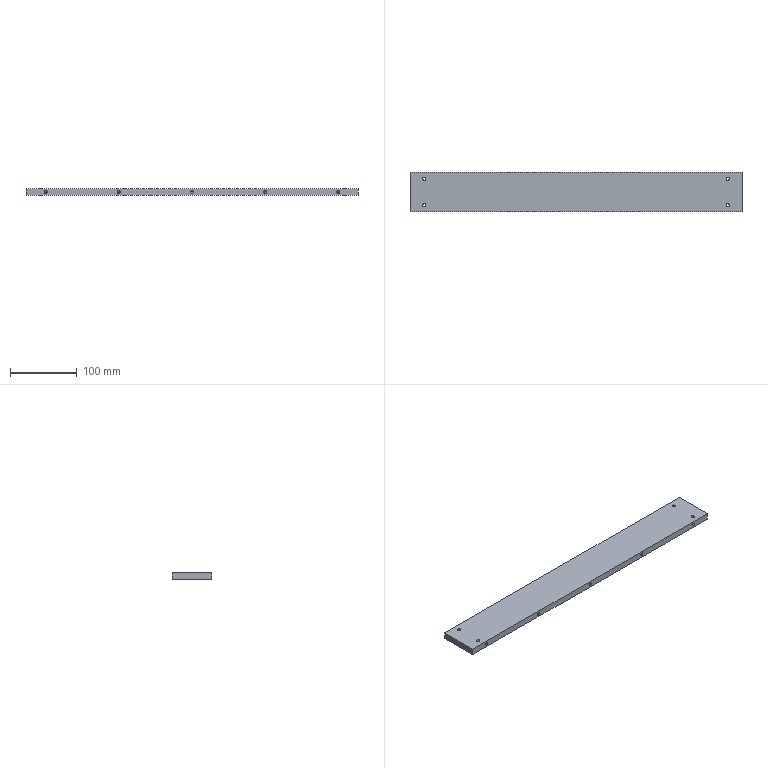Part | SolidWorks | features HoleWzd 3, Extrusion 1 | 1 solid | 54 faces | box 499 x 60 x 10 mm | volume 297280 mm3 | cylinder 28 | cone 20 | plane 6 | commonest cylinder face diameters 3.3 x10 4.2 x10 5 x8
STEP:
#1=CARTESIAN_POINT('',(0.,49.9,-1.65));
#2=VERTEX_POINT('',#1);
#3=CARTESIAN_POINT('',(0.,49.9,1.65));
#4=VERTEX_POINT('',#3);
#5=CARTESIAN_POINT('',(0.,49.9,0.));
#6=DIRECTION('',(0.,1.,0.));
#7=DIRECTION('',(0.,0.,1.));
#8=AXIS2_PLACEMENT_3D('',#5,#6,#7);
#9=CIRCLE('',#8,1.65);
#10=EDGE_CURVE('',#2,#4,#9,.T.);
#11=ORIENTED_EDGE('',*,*,#10,.F.);
#12=CARTESIAN_POINT('',(0.,60.,-1.65));
#13=VERTEX_POINT('',#12);
#14=CARTESIAN_POINT('',(0.,60.,-1.65));
#15=DIRECTION('',(0.,1.,0.));
#16=VECTOR('',#15,1000.);
#17=LINE('',#14,#16);
#18=EDGE_CURVE('',#2,#13,#17,.T.);
#19=ORIENTED_EDGE('',*,*,#18,.T.);
#20=CARTESIAN_POINT('',(0.,60.,1.65));
#21=VERTEX_POINT('',#20);
#22=CARTESIAN_POINT('',(0.,60.,0.));
#23=DIRECTION('',(0.,1.,0.));
#24=DIRECTION('',(0.,0.,1.));
#25=AXIS2_PLACEMENT_3D('',#22,#23,#24);
#26=CIRCLE('',#25,1.65);
#27=EDGE_CURVE('',#13,#21,#26,.T.);
#28=ORIENTED_EDGE('',*,*,#27,.T.);
#29=CARTESIAN_POINT('',(0.,60.,1.65));
#30=DIRECTION('',(0.,1.,0.));
#31=VECTOR('',#30,1000.);
#32=LINE('',#29,#31);
#33=EDGE_CURVE('',#4,#21,#32,.T.);
#34=ORIENTED_EDGE('',*,*,#33,.F.);
#35=EDGE_LOOP('',(#11,#19,#28,#34));
#36=FACE_OUTER_BOUND('',#35,.T.);
#37=CARTESIAN_POINT('',(0.,60.,0.));
#38=DIRECTION('',(0.,1.,0.));
#39=DIRECTION('',(0.,0.,1.));
#40=AXIS2_PLACEMENT_3D('',#37,#38,#39);
#41=CYLINDRICAL_SURFACE('',#40,1.65);
#42=ADVANCED_FACE('',(#36),#41,.F.);
#43=CARTESIAN_POINT('',(0.,48.909,0.));
#44=VERTEX_POINT('',#43);
#45=CARTESIAN_POINT('',(0.,49.9,1.65));
#46=DIRECTION('',(0.,0.515,0.8572));
#47=VECTOR('',#46,1000.);
#48=LINE('',#45,#47);
#49=EDGE_CURVE('',#44,#4,#48,.T.);
#50=ORIENTED_EDGE('',*,*,#49,.F.);
#51=CARTESIAN_POINT('',(0.,49.9,-1.65));
#52=DIRECTION('',(0.,0.515,-0.8572));
#53=VECTOR('',#52,1000.);
#54=LINE('',#51,#53);
#55=EDGE_CURVE('',#44,#2,#54,.T.);
#56=ORIENTED_EDGE('',*,*,#55,.T.);
#57=ORIENTED_EDGE('',*,*,#10,.T.);
#58=EDGE_LOOP('',(#50,#56,#57));
#59=FACE_OUTER_BOUND('',#58,.T.);
#60=CARTESIAN_POINT('',(0.,49.9,0.));
#61=DIRECTION('',(0.,1.,0.));
#62=DIRECTION('',(0.,0.,1.));
#63=AXIS2_PLACEMENT_3D('',#60,#61,#62);
#64=CONICAL_SURFACE('',#63,1.65,1.03);
#65=ADVANCED_FACE('',(#59),#64,.F.);
#66=CARTESIAN_POINT('',(-175.,49.9,-1.65));
#67=VERTEX_POINT('',#66);
#68=CARTESIAN_POINT('',(-175.,49.9,1.65));
#69=VERTEX_POINT('',#68);
#70=CARTESIAN_POINT('',(-175.,49.9,0.));
#71=DIRECTION('',(0.,1.,0.));
#72=DIRECTION('',(0.,0.,1.));
#73=AXIS2_PLACEMENT_3D('',#70,#71,#72);
#74=CIRCLE('',#73,1.65);
#75=EDGE_CURVE('',#67,#69,#74,.T.);
#76=ORIENTED_EDGE('',*,*,#75,.F.);
#77=CARTESIAN_POINT('',(-175.,60.,-1.65));
#78=VERTEX_POINT('',#77);
#79=CARTESIAN_POINT('',(-175.,60.,-1.65));
#80=DIRECTION('',(0.,1.,0.));
#81=VECTOR('',#80,1000.);
#82=LINE('',#79,#81);
#83=EDGE_CURVE('',#67,#78,#82,.T.);
#84=ORIENTED_EDGE('',*,*,#83,.T.);
#85=CARTESIAN_POINT('',(-175.,60.,1.65));
#86=VERTEX_POINT('',#85);
#87=CARTESIAN_POINT('',(-175.,60.,0.));
#88=DIRECTION('',(0.,1.,0.));
#89=DIRECTION('',(0.,0.,1.));
#90=AXIS2_PLACEMENT_3D('',#87,#88,#89);
#91=CIRCLE('',#90,1.65);
#92=EDGE_CURVE('',#78,#86,#91,.T.);
#93=ORIENTED_EDGE('',*,*,#92,.T.);
#94=CARTESIAN_POINT('',(-175.,60.,1.65));
#95=DIRECTION('',(0.,1.,0.));
#96=VECTOR('',#95,1000.);
#97=LINE('',#94,#96);
#98=EDGE_CURVE('',#69,#86,#97,.T.);
#99=ORIENTED_EDGE('',*,*,#98,.F.);
#100=EDGE_LOOP('',(#76,#84,#93,#99));
#101=FACE_OUTER_BOUND('',#100,.T.);
#102=CARTESIAN_POINT('',(-175.,60.,0.));
#103=DIRECTION('',(0.,1.,0.));
#104=DIRECTION('',(0.,0.,1.));
#105=AXIS2_PLACEMENT_3D('',#102,#103,#104);
#106=CYLINDRICAL_SURFACE('',#105,1.65);
#107=ADVANCED_FACE('',(#101),#106,.F.);
#108=CARTESIAN_POINT('',(-175.,48.909,0.));
#109=VERTEX_POINT('',#108);
#110=CARTESIAN_POINT('',(-175.,49.9,1.65));
#111=DIRECTION('',(0.,0.515,0.8572));
#112=VECTOR('',#111,1000.);
#113=LINE('',#110,#112);
#114=EDGE_CURVE('',#109,#69,#113,.T.);
#115=ORIENTED_EDGE('',*,*,#114,.F.);
#116=CARTESIAN_POINT('',(-175.,49.9,-1.65));
#117=DIRECTION('',(0.,0.515,-0.8572));
#118=VECTOR('',#117,1000.);
#119=LINE('',#116,#118);
#120=EDGE_CURVE('',#109,#67,#119,.T.);
#121=ORIENTED_EDGE('',*,*,#120,.T.);
#122=ORIENTED_EDGE('',*,*,#75,.T.);
#123=EDGE_LOOP('',(#115,#121,#122));
#124=FACE_OUTER_BOUND('',#123,.T.);
#125=CARTESIAN_POINT('',(-175.,49.9,0.));
#126=DIRECTION('',(0.,1.,0.));
#127=DIRECTION('',(0.,0.,1.));
#128=AXIS2_PLACEMENT_3D('',#125,#126,#127);
#129=CONICAL_SURFACE('',#128,1.65,1.03);
#130=ADVANCED_FACE('',(#124),#129,.F.);
#131=CARTESIAN_POINT('',(175.,49.9,-1.65));
#132=VERTEX_POINT('',#131);
#133=CARTESIAN_POINT('',(175.,49.9,1.65));
#134=VERTEX_POINT('',#133);
#135=CARTESIAN_POINT('',(175.,49.9,0.));
#136=DIRECTION('',(0.,1.,0.));
#137=DIRECTION('',(0.,0.,1.));
#138=AXIS2_PLACEMENT_3D('',#135,#136,#137);
#139=CIRCLE('',#138,1.65);
#140=EDGE_CURVE('',#132,#134,#139,.T.);
#141=ORIENTED_EDGE('',*,*,#140,.F.);
#142=CARTESIAN_POINT('',(175.,60.,-1.65));
#143=VERTEX_POINT('',#142);
#144=CARTESIAN_POINT('',(175.,60.,-1.65));
#145=DIRECTION('',(0.,1.,0.));
#146=VECTOR('',#145,1000.);
#147=LINE('',#144,#146);
#148=EDGE_CURVE('',#132,#143,#147,.T.);
#149=ORIENTED_EDGE('',*,*,#148,.T.);
#150=CARTESIAN_POINT('',(175.,60.,1.65));
#151=VERTEX_POINT('',#150);
#152=CARTESIAN_POINT('',(175.,60.,0.));
#153=DIRECTION('',(0.,1.,0.));
#154=DIRECTION('',(0.,0.,1.));
#155=AXIS2_PLACEMENT_3D('',#152,#153,#154);
#156=CIRCLE('',#155,1.65);
#157=EDGE_CURVE('',#143,#151,#156,.T.);
#158=ORIENTED_EDGE('',*,*,#157,.T.);
#159=CARTESIAN_POINT('',(175.,60.,1.65));
#160=DIRECTION('',(0.,1.,0.));
#161=VECTOR('',#160,1000.);
#162=LINE('',#159,#161);
#163=EDGE_CURVE('',#134,#151,#162,.T.);
#164=ORIENTED_EDGE('',*,*,#163,.F.);
#165=EDGE_LOOP('',(#141,#149,#158,#164));
#166=FACE_OUTER_BOUND('',#165,.T.);
#167=CARTESIAN_POINT('',(175.,60.,0.));
#168=DIRECTION('',(0.,1.,0.));
#169=DIRECTION('',(0.,0.,1.));
#170=AXIS2_PLACEMENT_3D('',#167,#168,#169);
#171=CYLINDRICAL_SURFACE('',#170,1.65);
#172=ADVANCED_FACE('',(#166),#171,.F.);
#173=CARTESIAN_POINT('',(175.,48.909,0.));
#174=VERTEX_POINT('',#173);
#175=CARTESIAN_POINT('',(175.,49.9,1.65));
#176=DIRECTION('',(0.,0.515,0.8572));
#177=VECTOR('',#176,1000.);
#178=LINE('',#175,#177);
#179=EDGE_CURVE('',#174,#134,#178,.T.);
#180=ORIENTED_EDGE('',*,*,#179,.F.);
#181=CARTESIAN_POINT('',(175.,49.9,-1.65));
#182=DIRECTION('',(0.,0.515,-0.8572));
#183=VECTOR('',#182,1000.);
#184=LINE('',#181,#183);
#185=EDGE_CURVE('',#174,#132,#184,.T.);
#186=ORIENTED_EDGE('',*,*,#185,.T.);
#187=ORIENTED_EDGE('',*,*,#140,.T.);
#188=EDGE_LOOP('',(#180,#186,#187));
#189=FACE_OUTER_BOUND('',#188,.T.);
#190=CARTESIAN_POINT('',(175.,49.9,0.));
#191=DIRECTION('',(0.,1.,0.));
#192=DIRECTION('',(0.,0.,1.));
#193=AXIS2_PLACEMENT_3D('',#190,#191,#192);
#194=CONICAL_SURFACE('',#193,1.65,1.03);
#195=ADVANCED_FACE('',(#189),#194,.F.);
#196=CARTESIAN_POINT('',(-160.,49.9,-1.65));
#197=VERTEX_POINT('',#196);
#198=CARTESIAN_POINT('',(-160.,49.9,1.65));
#199=VERTEX_POINT('',#198);
#200=CARTESIAN_POINT('',(-160.,49.9,0.));
#201=DIRECTION('',(0.,1.,0.));
#202=DIRECTION('',(0.,0.,1.));
#203=AXIS2_PLACEMENT_3D('',#200,#201,#202);
#204=CIRCLE('',#203,1.65);
#205=EDGE_CURVE('',#197,#199,#204,.T.);
#206=ORIENTED_EDGE('',*,*,#205,.F.);
#207=CARTESIAN_POINT('',(-160.,60.,-1.65));
#208=VERTEX_POINT('',#207);
#209=CARTESIAN_POINT('',(-160.,60.,-1.65));
#210=DIRECTION('',(0.,1.,0.));
#211=VECTOR('',#210,1000.);
#212=LINE('',#209,#211);
#213=EDGE_CURVE('',#197,#208,#212,.T.);
#214=ORIENTED_EDGE('',*,*,#213,.T.);
#215=CARTESIAN_POINT('',(-160.,60.,1.65));
#216=VERTEX_POINT('',#215);
#217=CARTESIAN_POINT('',(-160.,60.,0.));
#218=DIRECTION('',(0.,1.,0.));
#219=DIRECTION('',(0.,0.,1.));
#220=AXIS2_PLACEMENT_3D('',#217,#218,#219);
#221=CIRCLE('',#220,1.65);
#222=EDGE_CURVE('',#208,#216,#221,.T.);
#223=ORIENTED_EDGE('',*,*,#222,.T.);
#224=CARTESIAN_POINT('',(-160.,60.,1.65));
#225=DIRECTION('',(0.,1.,0.));
#226=VECTOR('',#225,1000.);
#227=LINE('',#224,#226);
#228=EDGE_CURVE('',#199,#216,#227,.T.);
#229=ORIENTED_EDGE('',*,*,#228,.F.);
#230=EDGE_LOOP('',(#206,#214,#223,#229));
#231=FACE_OUTER_BOUND('',#230,.T.);
#232=CARTESIAN_POINT('',(-160.,60.,0.));
#233=DIRECTION('',(0.,1.,0.));
#234=DIRECTION('',(0.,0.,1.));
#235=AXIS2_PLACEMENT_3D('',#232,#233,#234);
#236=CYLINDRICAL_SURFACE('',#235,1.65);
#237=ADVANCED_FACE('',(#231),#236,.F.);
#238=CARTESIAN_POINT('',(-160.,48.909,0.));
#239=VERTEX_POINT('',#238);
#240=CARTESIAN_POINT('',(-160.,49.9,1.65));
#241=DIRECTION('',(0.,0.515,0.8572));
#242=VECTOR('',#241,1000.);
#243=LINE('',#240,#242);
#244=EDGE_CURVE('',#239,#199,#243,.T.);
#245=ORIENTED_EDGE('',*,*,#244,.F.);
#246=CARTESIAN_POINT('',(-160.,49.9,-1.65));
#247=DIRECTION('',(0.,0.515,-0.8572));
#248=VECTOR('',#247,1000.);
#249=LINE('',#246,#248);
#250=EDGE_CURVE('',#239,#197,#249,.T.);
#251=ORIENTED_EDGE('',*,*,#250,.T.);
#252=ORIENTED_EDGE('',*,*,#205,.T.);
#253=EDGE_LOOP('',(#245,#251,#252));
#254=FACE_OUTER_BOUND('',#253,.T.);
#255=CARTESIAN_POINT('',(-160.,49.9,0.));
#256=DIRECTION('',(0.,1.,0.));
#257=DIRECTION('',(0.,0.,1.));
#258=AXIS2_PLACEMENT_3D('',#255,#256,#257);
#259=CONICAL_SURFACE('',#258,1.65,1.03);
#260=ADVANCED_FACE('',(#254),#259,.F.);
#261=CARTESIAN_POINT('',(160.,49.9,-1.65));
#262=VERTEX_POINT('',#261);
#263=CARTESIAN_POINT('',(160.,49.9,1.65));
#264=VERTEX_POINT('',#263);
#265=CARTESIAN_POINT('',(160.,49.9,0.));
#266=DIRECTION('',(0.,1.,0.));
#267=DIRECTION('',(0.,0.,1.));
#268=AXIS2_PLACEMENT_3D('',#265,#266,#267);
#269=CIRCLE('',#268,1.65);
#270=EDGE_CURVE('',#262,#264,#269,.T.);
#271=ORIENTED_EDGE('',*,*,#270,.F.);
#272=CARTESIAN_POINT('',(160.,60.,-1.65));
#273=VERTEX_POINT('',#272);
#274=CARTESIAN_POINT('',(160.,60.,-1.65));
#275=DIRECTION('',(0.,1.,0.));
#276=VECTOR('',#275,1000.);
#277=LINE('',#274,#276);
#278=EDGE_CURVE('',#262,#273,#277,.T.);
#279=ORIENTED_EDGE('',*,*,#278,.T.);
#280=CARTESIAN_POINT('',(160.,60.,1.65));
#281=VERTEX_POINT('',#280);
#282=CARTESIAN_POINT('',(160.,60.,0.));
#283=DIRECTION('',(0.,1.,0.));
#284=DIRECTION('',(0.,0.,1.));
#285=AXIS2_PLACEMENT_3D('',#282,#283,#284);
#286=CIRCLE('',#285,1.65);
#287=EDGE_CURVE('',#273,#281,#286,.T.);
#288=ORIENTED_EDGE('',*,*,#287,.T.);
#289=CARTESIAN_POINT('',(160.,60.,1.65));
#290=DIRECTION('',(0.,1.,0.));
#291=VECTOR('',#290,1000.);
#292=LINE('',#289,#291);
#293=EDGE_CURVE('',#264,#281,#292,.T.);
#294=ORIENTED_EDGE('',*,*,#293,.F.);
#295=EDGE_LOOP('',(#271,#279,#288,#294));
#296=FACE_OUTER_BOUND('',#295,.T.);
#297=CARTESIAN_POINT('',(160.,60.,0.));
#298=DIRECTION('',(0.,1.,0.));
#299=DIRECTION('',(0.,0.,1.));
#300=AXIS2_PLACEMENT_3D('',#297,#298,#299);
#301=CYLINDRICAL_SURFACE('',#300,1.65);
#302=ADVANCED_FACE('',(#296),#301,.F.);
#303=CARTESIAN_POINT('',(160.,48.909,0.));
#304=VERTEX_POINT('',#303);
#305=CARTESIAN_POINT('',(160.,49.9,1.65));
#306=DIRECTION('',(0.,0.515,0.8572));
#307=VECTOR('',#306,1000.);
#308=LINE('',#305,#307);
#309=EDGE_CURVE('',#304,#264,#308,.T.);
#310=ORIENTED_EDGE('',*,*,#309,.F.);
#311=CARTESIAN_POINT('',(160.,49.9,-1.65));
#312=DIRECTION('',(0.,0.515,-0.8572));
#313=VECTOR('',#312,1000.);
#314=LINE('',#311,#313);
#315=EDGE_CURVE('',#304,#262,#314,.T.);
#316=ORIENTED_EDGE('',*,*,#315,.T.);
#317=ORIENTED_EDGE('',*,*,#270,.T.);
#318=EDGE_LOOP('',(#310,#316,#317));
#319=FACE_OUTER_BOUND('',#318,.T.);
#320=CARTESIAN_POINT('',(160.,49.9,0.));
#321=DIRECTION('',(0.,1.,0.));
#322=DIRECTION('',(0.,0.,1.));
#323=AXIS2_PLACEMENT_3D('',#320,#321,#322);
#324=CONICAL_SURFACE('',#323,1.65,1.03);
#325=ADVANCED_FACE('',(#319),#324,.F.);
#326=CARTESIAN_POINT('',(225.5,50.,-5.));
#327=VERTEX_POINT('',#326);
#328=CARTESIAN_POINT('',(230.5,50.,-5.));
#329=VERTEX_POINT('',#328);
#330=CARTESIAN_POINT('',(228.,50.,-5.));
#331=DIRECTION('',(0.,0.,1.));
#332=DIRECTION('',(1.,0.,0.));
#333=AXIS2_PLACEMENT_3D('',#330,#331,#332);
#334=CIRCLE('',#333,2.5);
#335=EDGE_CURVE('',#327,#329,#334,.T.);
#336=ORIENTED_EDGE('',*,*,#335,.F.);
#337=CARTESIAN_POINT('',(225.5,50.,5.));
#338=VERTEX_POINT('',#337);
#339=CARTESIAN_POINT('',(225.5,50.,5.));
#340=DIRECTION('',(0.,0.,1.));
#341=VECTOR('',#340,1000.);
#342=LINE('',#339,#341);
#343=EDGE_CURVE('',#327,#338,#342,.T.);
#344=ORIENTED_EDGE('',*,*,#343,.T.);
#345=CARTESIAN_POINT('',(230.5,50.,5.));
#346=VERTEX_POINT('',#345);
#347=CARTESIAN_POINT('',(228.,50.,5.));
#348=DIRECTION('',(0.,0.,1.));
#349=DIRECTION('',(1.,0.,0.));
#350=AXIS2_PLACEMENT_3D('',#347,#348,#349);
#351=CIRCLE('',#350,2.5);
#352=EDGE_CURVE('',#338,#346,#351,.T.);
#353=ORIENTED_EDGE('',*,*,#352,.T.);
#354=CARTESIAN_POINT('',(230.5,50.,5.));
#355=DIRECTION('',(0.,0.,1.));
#356=VECTOR('',#355,1000.);
#357=LINE('',#354,#356);
#358=EDGE_CURVE('',#329,#346,#357,.T.);
#359=ORIENTED_EDGE('',*,*,#358,.F.);
#360=EDGE_LOOP('',(#336,#344,#353,#359));
#361=FACE_OUTER_BOUND('',#360,.T.);
#362=CARTESIAN_POINT('',(228.,50.,5.));
#363=DIRECTION('',(0.,0.,1.));
#364=DIRECTION('',(1.,0.,0.));
#365=AXIS2_PLACEMENT_3D('',#362,#363,#364);
#366=CYLINDRICAL_SURFACE('',#365,2.5);
#367=ADVANCED_FACE('',(#361),#366,.F.);
#368=CARTESIAN_POINT('',(225.5,10.,-5.));
#369=VERTEX_POINT('',#368);
#370=CARTESIAN_POINT('',(230.5,10.,-5.));
#371=VERTEX_POINT('',#370);
#372=CARTESIAN_POINT('',(228.,10.,-5.));
#373=DIRECTION('',(0.,0.,1.));
#374=DIRECTION('',(1.,0.,0.));
#375=AXIS2_PLACEMENT_3D('',#372,#373,#374);
#376=CIRCLE('',#375,2.5);
#377=EDGE_CURVE('',#369,#371,#376,.T.);
#378=ORIENTED_EDGE('',*,*,#377,.F.);
#379=CARTESIAN_POINT('',(225.5,10.,5.));
#380=VERTEX_POINT('',#379);
#381=CARTESIAN_POINT('',(225.5,10.,5.));
#382=DIRECTION('',(0.,0.,1.));
#383=VECTOR('',#382,1000.);
#384=LINE('',#381,#383);
#385=EDGE_CURVE('',#369,#380,#384,.T.);
#386=ORIENTED_EDGE('',*,*,#385,.T.);
#387=CARTESIAN_POINT('',(230.5,10.,5.));
#388=VERTEX_POINT('',#387);
#389=CARTESIAN_POINT('',(228.,10.,5.));
#390=DIRECTION('',(0.,0.,1.));
#391=DIRECTION('',(1.,0.,0.));
#392=AXIS2_PLACEMENT_3D('',#389,#390,#391);
#393=CIRCLE('',#392,2.5);
#394=EDGE_CURVE('',#380,#388,#393,.T.);
#395=ORIENTED_EDGE('',*,*,#394,.T.);
#396=CARTESIAN_POINT('',(230.5,10.,5.));
#397=DIRECTION('',(0.,0.,1.));
#398=VECTOR('',#397,1000.);
#399=LINE('',#396,#398);
#400=EDGE_CURVE('',#371,#388,#399,.T.);
#401=ORIENTED_EDGE('',*,*,#400,.F.);
#402=EDGE_LOOP('',(#378,#386,#395,#401));
#403=FACE_OUTER_BOUND('',#402,.T.);
#404=CARTESIAN_POINT('',(228.,10.,5.));
#405=DIRECTION('',(0.,0.,1.));
#406=DIRECTION('',(1.,0.,0.));
#407=AXIS2_PLACEMENT_3D('',#404,#405,#406);
#408=CYLINDRICAL_SURFACE('',#407,2.5);
#409=ADVANCED_FACE('',(#403),#408,.F.);
#410=CARTESIAN_POINT('',(-230.5,10.,-5.));
#411=VERTEX_POINT('',#410);
#412=CARTESIAN_POINT('',(-225.5,10.,-5.));
#413=VERTEX_POINT('',#412);
#414=CARTESIAN_POINT('',(-228.,10.,-5.));
#415=DIRECTION('',(0.,0.,1.));
#416=DIRECTION('',(1.,0.,0.));
#417=AXIS2_PLACEMENT_3D('',#414,#415,#416);
#418=CIRCLE('',#417,2.5);
#419=EDGE_CURVE('',#411,#413,#418,.T.);
#420=ORIENTED_EDGE('',*,*,#419,.F.);
#421=CARTESIAN_POINT('',(-230.5,10.,5.));
#422=VERTEX_POINT('',#421);
#423=CARTESIAN_POINT('',(-230.5,10.,5.));
#424=DIRECTION('',(0.,0.,1.));
#425=VECTOR('',#424,1000.);
#426=LINE('',#423,#425);
#427=EDGE_CURVE('',#411,#422,#426,.T.);
#428=ORIENTED_EDGE('',*,*,#427,.T.);
#429=CARTESIAN_POINT('',(-225.5,10.,5.));
#430=VERTEX_POINT('',#429);
#431=CARTESIAN_POINT('',(-228.,10.,5.));
#432=DIRECTION('',(0.,0.,1.));
#433=DIRECTION('',(1.,0.,0.));
#434=AXIS2_PLACEMENT_3D('',#431,#432,#433);
#435=CIRCLE('',#434,2.5);
#436=EDGE_CURVE('',#422,#430,#435,.T.);
#437=ORIENTED_EDGE('',*,*,#436,.T.);
#438=CARTESIAN_POINT('',(-225.5,10.,5.));
#439=DIRECTION('',(0.,0.,1.));
#440=VECTOR('',#439,1000.);
#441=LINE('',#438,#440);
#442=EDGE_CURVE('',#413,#430,#441,.T.);
#443=ORIENTED_EDGE('',*,*,#442,.F.);
#444=EDGE_LOOP('',(#420,#428,#437,#443));
#445=FACE_OUTER_BOUND('',#444,.T.);
#446=CARTESIAN_POINT('',(-228.,10.,5.));
#447=DIRECTION('',(0.,0.,1.));
#448=DIRECTION('',(1.,0.,0.));
#449=AXIS2_PLACEMENT_3D('',#446,#447,#448);
#450=CYLINDRICAL_SURFACE('',#449,2.5);
#451=ADVANCED_FACE('',(#445),#450,.F.);
#452=CARTESIAN_POINT('',(-230.5,50.,-5.));
#453=VERTEX_POINT('',#452);
#454=CARTESIAN_POINT('',(-225.5,50.,-5.));
#455=VERTEX_POINT('',#454);
#456=CARTESIAN_POINT('',(-228.,50.,-5.));
#457=DIRECTION('',(0.,0.,1.));
#458=DIRECTION('',(1.,0.,0.));
#459=AXIS2_PLACEMENT_3D('',#456,#457,#458);
#460=CIRCLE('',#459,2.5);
#461=EDGE_CURVE('',#453,#455,#460,.T.);
#462=ORIENTED_EDGE('',*,*,#461,.F.);
#463=CARTESIAN_POINT('',(-230.5,50.,5.));
#464=VERTEX_POINT('',#463);
#465=CARTESIAN_POINT('',(-230.5,50.,5.));
#466=DIRECTION('',(0.,0.,1.));
#467=VECTOR('',#466,1000.);
#468=LINE('',#465,#467);
#469=EDGE_CURVE('',#453,#464,#468,.T.);
#470=ORIENTED_EDGE('',*,*,#469,.T.);
#471=CARTESIAN_POINT('',(-225.5,50.,5.));
#472=VERTEX_POINT('',#471);
#473=CARTESIAN_POINT('',(-228.,50.,5.));
#474=DIRECTION('',(0.,0.,1.));
#475=DIRECTION('',(1.,0.,0.));
#476=AXIS2_PLACEMENT_3D('',#473,#474,#475);
#477=CIRCLE('',#476,2.5);
#478=EDGE_CURVE('',#464,#472,#477,.T.);
#479=ORIENTED_EDGE('',*,*,#478,.T.);
#480=CARTESIAN_POINT('',(-225.5,50.,5.));
#481=DIRECTION('',(0.,0.,1.));
#482=VECTOR('',#481,1000.);
#483=LINE('',#480,#482);
#484=EDGE_CURVE('',#455,#472,#483,.T.);
#485=ORIENTED_EDGE('',*,*,#484,.F.);
#486=EDGE_LOOP('',(#462,#470,#479,#485));
#487=FACE_OUTER_BOUND('',#486,.T.);
#488=CARTESIAN_POINT('',(-228.,50.,5.));
#489=DIRECTION('',(0.,0.,1.));
#490=DIRECTION('',(1.,0.,0.));
#491=AXIS2_PLACEMENT_3D('',#488,#489,#490);
#492=CYLINDRICAL_SURFACE('',#491,2.5);
#493=ADVANCED_FACE('',(#487),#492,.F.);
#494=CARTESIAN_POINT('',(220.,12.4,2.1));
#495=VERTEX_POINT('',#494);
#496=CARTESIAN_POINT('',(220.,12.4,-2.1));
#497=VERTEX_POINT('',#496);
#498=CARTESIAN_POINT('',(220.,12.4,0.));
#499=DIRECTION('',(0.,-1.,0.));
#500=DIRECTION('',(0.,0.,-1.));
#501=AXIS2_PLACEMENT_3D('',#498,#499,#500);
#502=CIRCLE('',#501,2.1);
#503=EDGE_CURVE('',#495,#497,#502,.T.);
#504=ORIENTED_EDGE('',*,*,#503,.F.);
#505=CARTESIAN_POINT('',(220.,0.,2.1));
#506=VERTEX_POINT('',#505);
#507=CARTESIAN_POINT('',(220.,0.,2.1));
#508=DIRECTION('',(0.,-1.,0.));
#509=VECTOR('',#508,1000.);
#510=LINE('',#507,#509);
#511=EDGE_CURVE('',#495,#506,#510,.T.);
#512=ORIENTED_EDGE('',*,*,#511,.T.);
#513=CARTESIAN_POINT('',(220.,0.,-2.1));
#514=VERTEX_POINT('',#513);
#515=CARTESIAN_POINT('',(220.,0.,0.));
#516=DIRECTION('',(0.,-1.,0.));
#517=DIRECTION('',(0.,0.,-1.));
#518=AXIS2_PLACEMENT_3D('',#515,#516,#517);
#519=CIRCLE('',#518,2.1);
#520=EDGE_CURVE('',#506,#514,#519,.T.);
#521=ORIENTED_EDGE('',*,*,#520,.T.);
#522=CARTESIAN_POINT('',(220.,0.,-2.1));
#523=DIRECTION('',(0.,-1.,0.));
#524=VECTOR('',#523,1000.);
#525=LINE('',#522,#524);
#526=EDGE_CURVE('',#497,#514,#525,.T.);
#527=ORIENTED_EDGE('',*,*,#526,.F.);
#528=EDGE_LOOP('',(#504,#512,#521,#527));
#529=FACE_OUTER_BOUND('',#528,.T.);
#530=CARTESIAN_POINT('',(220.,0.,0.));
#531=DIRECTION('',(0.,-1.,0.));
#532=DIRECTION('',(0.,0.,-1.));
#533=AXIS2_PLACEMENT_3D('',#530,#531,#532);
#534=CYLINDRICAL_SURFACE('',#533,2.1);
#535=ADVANCED_FACE('',(#529),#534,.F.);
#536=CARTESIAN_POINT('',(220.,13.662,0.));
#537=VERTEX_POINT('',#536);
#538=CARTESIAN_POINT('',(220.,12.4,-2.1));
#539=DIRECTION('',(0.,-0.515,-0.8572));
#540=VECTOR('',#539,1000.);
#541=LINE('',#538,#540);
#542=EDGE_CURVE('',#537,#497,#541,.T.);
#543=ORIENTED_EDGE('',*,*,#542,.F.);
#544=CARTESIAN_POINT('',(220.,12.4,2.1));
#545=DIRECTION('',(0.,-0.515,0.8572));
#546=VECTOR('',#545,1000.);
#547=LINE('',#544,#546);
#548=EDGE_CURVE('',#537,#495,#547,.T.);
#549=ORIENTED_EDGE('',*,*,#548,.T.);
#550=ORIENTED_EDGE('',*,*,#503,.T.);
#551=EDGE_LOOP('',(#543,#549,#550));
#552=FACE_OUTER_BOUND('',#551,.T.);
#553=CARTESIAN_POINT('',(220.,12.4,0.));
#554=DIRECTION('',(0.,-1.,0.));
#555=DIRECTION('',(0.,0.,-1.));
#556=AXIS2_PLACEMENT_3D('',#553,#554,#555);
#557=CONICAL_SURFACE('',#556,2.1,1.03);
#558=ADVANCED_FACE('',(#552),#557,.F.);
#559=CARTESIAN_POINT('',(110.,12.4,2.1));
#560=VERTEX_POINT('',#559);
#561=CARTESIAN_POINT('',(110.,12.4,-2.1));
#562=VERTEX_POINT('',#561);
#563=CARTESIAN_POINT('',(110.,12.4,0.));
#564=DIRECTION('',(0.,-1.,0.));
#565=DIRECTION('',(0.,0.,-1.));
#566=AXIS2_PLACEMENT_3D('',#563,#564,#565);
#567=CIRCLE('',#566,2.1);
#568=EDGE_CURVE('',#560,#562,#567,.T.);
#569=ORIENTED_EDGE('',*,*,#568,.F.);
#570=CARTESIAN_POINT('',(110.,0.,2.1));
#571=VERTEX_POINT('',#570);
#572=CARTESIAN_POINT('',(110.,0.,2.1));
#573=DIRECTION('',(0.,-1.,0.));
#574=VECTOR('',#573,1000.);
#575=LINE('',#572,#574);
#576=EDGE_CURVE('',#560,#571,#575,.T.);
#577=ORIENTED_EDGE('',*,*,#576,.T.);
#578=CARTESIAN_POINT('',(110.,0.,-2.1));
#579=VERTEX_POINT('',#578);
#580=CARTESIAN_POINT('',(110.,0.,0.));
#581=DIRECTION('',(0.,-1.,0.));
#582=DIRECTION('',(0.,0.,-1.));
#583=AXIS2_PLACEMENT_3D('',#580,#581,#582);
#584=CIRCLE('',#583,2.1);
#585=EDGE_CURVE('',#571,#579,#584,.T.);
#586=ORIENTED_EDGE('',*,*,#585,.T.);
#587=CARTESIAN_POINT('',(110.,0.,-2.1));
#588=DIRECTION('',(0.,-1.,0.));
#589=VECTOR('',#588,1000.);
#590=LINE('',#587,#589);
#591=EDGE_CURVE('',#562,#579,#590,.T.);
#592=ORIENTED_EDGE('',*,*,#591,.F.);
#593=EDGE_LOOP('',(#569,#577,#586,#592));
#594=FACE_OUTER_BOUND('',#593,.T.);
#595=CARTESIAN_POINT('',(110.,0.,0.));
#596=DIRECTION('',(0.,-1.,0.));
#597=DIRECTION('',(0.,0.,-1.));
#598=AXIS2_PLACEMENT_3D('',#595,#596,#597);
#599=CYLINDRICAL_SURFACE('',#598,2.1);
#600=ADVANCED_FACE('',(#594),#599,.F.);
#601=CARTESIAN_POINT('',(110.,13.662,0.));
#602=VERTEX_POINT('',#601);
#603=CARTESIAN_POINT('',(110.,12.4,-2.1));
#604=DIRECTION('',(0.,-0.515,-0.8572));
#605=VECTOR('',#604,1000.);
#606=LINE('',#603,#605);
#607=EDGE_CURVE('',#602,#562,#606,.T.);
#608=ORIENTED_EDGE('',*,*,#607,.F.);
#609=CARTESIAN_POINT('',(110.,12.4,2.1));
#610=DIRECTION('',(0.,-0.515,0.8572));
#611=VECTOR('',#610,1000.);
#612=LINE('',#609,#611);
#613=EDGE_CURVE('',#602,#560,#612,.T.);
#614=ORIENTED_EDGE('',*,*,#613,.T.);
#615=ORIENTED_EDGE('',*,*,#568,.T.);
#616=EDGE_LOOP('',(#608,#614,#615));
#617=FACE_OUTER_BOUND('',#616,.T.);
#618=CARTESIAN_POINT('',(110.,12.4,0.));
#619=DIRECTION('',(0.,-1.,0.));
#620=DIRECTION('',(0.,0.,-1.));
#621=AXIS2_PLACEMENT_3D('',#618,#619,#620);
#622=CONICAL_SURFACE('',#621,2.1,1.03);
#623=ADVANCED_FACE('',(#617),#622,.F.);
#624=CARTESIAN_POINT('',(0.,12.4,2.1));
#625=VERTEX_POINT('',#624);
#626=CARTESIAN_POINT('',(0.,12.4,-2.1));
#627=VERTEX_POINT('',#626);
#628=CARTESIAN_POINT('',(0.,12.4,0.));
#629=DIRECTION('',(0.,-1.,0.));
#630=DIRECTION('',(0.,0.,-1.));
#631=AXIS2_PLACEMENT_3D('',#628,#629,#630);
#632=CIRCLE('',#631,2.1);
#633=EDGE_CURVE('',#625,#627,#632,.T.);
#634=ORIENTED_EDGE('',*,*,#633,.F.);
#635=CARTESIAN_POINT('',(0.,0.,2.1));
#636=VERTEX_POINT('',#635);
#637=CARTESIAN_POINT('',(0.,0.,2.1));
#638=DIRECTION('',(0.,-1.,0.));
#639=VECTOR('',#638,1000.);
#640=LINE('',#637,#639);
#641=EDGE_CURVE('',#625,#636,#640,.T.);
#642=ORIENTED_EDGE('',*,*,#641,.T.);
#643=CARTESIAN_POINT('',(0.,0.,-2.1));
#644=VERTEX_POINT('',#643);
#645=CARTESIAN_POINT('',(0.,0.,0.));
#646=DIRECTION('',(0.,-1.,0.));
#647=DIRECTION('',(0.,0.,-1.));
#648=AXIS2_PLACEMENT_3D('',#645,#646,#647);
#649=CIRCLE('',#648,2.1);
#650=EDGE_CURVE('',#636,#644,#649,.T.);
#651=ORIENTED_EDGE('',*,*,#650,.T.);
#652=CARTESIAN_POINT('',(0.,0.,-2.1));
#653=DIRECTION('',(0.,-1.,0.));
#654=VECTOR('',#653,1000.);
#655=LINE('',#652,#654);
#656=EDGE_CURVE('',#627,#644,#655,.T.);
#657=ORIENTED_EDGE('',*,*,#656,.F.);
#658=EDGE_LOOP('',(#634,#642,#651,#657));
#659=FACE_OUTER_BOUND('',#658,.T.);
#660=CARTESIAN_POINT('',(0.,0.,0.));
#661=DIRECTION('',(0.,-1.,0.));
#662=DIRECTION('',(0.,0.,-1.));
#663=AXIS2_PLACEMENT_3D('',#660,#661,#662);
#664=CYLINDRICAL_SURFACE('',#663,2.1);
#665=ADVANCED_FACE('',(#659),#664,.F.);
#666=CARTESIAN_POINT('',(0.,13.662,0.));
#667=VERTEX_POINT('',#666);
#668=CARTESIAN_POINT('',(0.,12.4,-2.1));
#669=DIRECTION('',(0.,-0.515,-0.8572));
#670=VECTOR('',#669,1000.);
#671=LINE('',#668,#670);
#672=EDGE_CURVE('',#667,#627,#671,.T.);
#673=ORIENTED_EDGE('',*,*,#672,.F.);
#674=CARTESIAN_POINT('',(0.,12.4,2.1));
#675=DIRECTION('',(0.,-0.515,0.8572));
#676=VECTOR('',#675,1000.);
#677=LINE('',#674,#676);
#678=EDGE_CURVE('',#667,#625,#677,.T.);
#679=ORIENTED_EDGE('',*,*,#678,.T.);
#680=ORIENTED_EDGE('',*,*,#633,.T.);
#681=EDGE_LOOP('',(#673,#679,#680));
#682=FACE_OUTER_BOUND('',#681,.T.);
#683=CARTESIAN_POINT('',(0.,12.4,0.));
#684=DIRECTION('',(0.,-1.,0.));
#685=DIRECTION('',(0.,0.,-1.));
#686=AXIS2_PLACEMENT_3D('',#683,#684,#685);
#687=CONICAL_SURFACE('',#686,2.1,1.03);
#688=ADVANCED_FACE('',(#682),#687,.F.);
#689=CARTESIAN_POINT('',(-110.,12.4,2.1));
#690=VERTEX_POINT('',#689);
#691=CARTESIAN_POINT('',(-110.,12.4,-2.1));
#692=VERTEX_POINT('',#691);
#693=CARTESIAN_POINT('',(-110.,12.4,0.));
#694=DIRECTION('',(0.,-1.,0.));
#695=DIRECTION('',(0.,0.,-1.));
#696=AXIS2_PLACEMENT_3D('',#693,#694,#695);
#697=CIRCLE('',#696,2.1);
#698=EDGE_CURVE('',#690,#692,#697,.T.);
#699=ORIENTED_EDGE('',*,*,#698,.F.);
#700=CARTESIAN_POINT('',(-110.,0.,2.1));
#701=VERTEX_POINT('',#700);
#702=CARTESIAN_POINT('',(-110.,0.,2.1));
#703=DIRECTION('',(0.,-1.,0.));
#704=VECTOR('',#703,1000.);
#705=LINE('',#702,#704);
#706=EDGE_CURVE('',#690,#701,#705,.T.);
#707=ORIENTED_EDGE('',*,*,#706,.T.);
#708=CARTESIAN_POINT('',(-110.,0.,-2.1));
#709=VERTEX_POINT('',#708);
#710=CARTESIAN_POINT('',(-110.,0.,0.));
#711=DIRECTION('',(0.,-1.,0.));
#712=DIRECTION('',(0.,0.,-1.));
#713=AXIS2_PLACEMENT_3D('',#710,#711,#712);
#714=CIRCLE('',#713,2.1);
#715=EDGE_CURVE('',#701,#709,#714,.T.);
#716=ORIENTED_EDGE('',*,*,#715,.T.);
#717=CARTESIAN_POINT('',(-110.,0.,-2.1));
#718=DIRECTION('',(0.,-1.,0.));
#719=VECTOR('',#718,1000.);
#720=LINE('',#717,#719);
#721=EDGE_CURVE('',#692,#709,#720,.T.);
#722=ORIENTED_EDGE('',*,*,#721,.F.);
#723=EDGE_LOOP('',(#699,#707,#716,#722));
#724=FACE_OUTER_BOUND('',#723,.T.);
#725=CARTESIAN_POINT('',(-110.,0.,0.));
#726=DIRECTION('',(0.,-1.,0.));
#727=DIRECTION('',(0.,0.,-1.));
#728=AXIS2_PLACEMENT_3D('',#725,#726,#727);
#729=CYLINDRICAL_SURFACE('',#728,2.1);
#730=ADVANCED_FACE('',(#724),#729,.F.);
#731=CARTESIAN_POINT('',(-110.,13.662,0.));
#732=VERTEX_POINT('',#731);
#733=CARTESIAN_POINT('',(-110.,12.4,-2.1));
#734=DIRECTION('',(0.,-0.515,-0.8572));
#735=VECTOR('',#734,1000.);
#736=LINE('',#733,#735);
#737=EDGE_CURVE('',#732,#692,#736,.T.);
#738=ORIENTED_EDGE('',*,*,#737,.F.);
#739=CARTESIAN_POINT('',(-110.,12.4,2.1));
#740=DIRECTION('',(0.,-0.515,0.8572));
#741=VECTOR('',#740,1000.);
#742=LINE('',#739,#741);
#743=EDGE_CURVE('',#732,#690,#742,.T.);
#744=ORIENTED_EDGE('',*,*,#743,.T.);
#745=ORIENTED_EDGE('',*,*,#698,.T.);
#746=EDGE_LOOP('',(#738,#744,#745));
#747=FACE_OUTER_BOUND('',#746,.T.);
#748=CARTESIAN_POINT('',(-110.,12.4,0.));
#749=DIRECTION('',(0.,-1.,0.));
#750=DIRECTION('',(0.,0.,-1.));
#751=AXIS2_PLACEMENT_3D('',#748,#749,#750);
#752=CONICAL_SURFACE('',#751,2.1,1.03);
#753=ADVANCED_FACE('',(#747),#752,.F.);
#754=CARTESIAN_POINT('',(-220.,12.4,2.1));
#755=VERTEX_POINT('',#754);
#756=CARTESIAN_POINT('',(-220.,12.4,-2.1));
#757=VERTEX_POINT('',#756);
#758=CARTESIAN_POINT('',(-220.,12.4,0.));
#759=DIRECTION('',(0.,-1.,0.));
#760=DIRECTION('',(0.,0.,-1.));
#761=AXIS2_PLACEMENT_3D('',#758,#759,#760);
#762=CIRCLE('',#761,2.1);
#763=EDGE_CURVE('',#755,#757,#762,.T.);
#764=ORIENTED_EDGE('',*,*,#763,.F.);
#765=CARTESIAN_POINT('',(-220.,0.,2.1));
#766=VERTEX_POINT('',#765);
#767=CARTESIAN_POINT('',(-220.,0.,2.1));
#768=DIRECTION('',(0.,-1.,0.));
#769=VECTOR('',#768,1000.);
#770=LINE('',#767,#769);
#771=EDGE_CURVE('',#755,#766,#770,.T.);
#772=ORIENTED_EDGE('',*,*,#771,.T.);
#773=CARTESIAN_POINT('',(-220.,0.,-2.1));
#774=VERTEX_POINT('',#773);
#775=CARTESIAN_POINT('',(-220.,0.,0.));
#776=DIRECTION('',(0.,-1.,0.));
#777=DIRECTION('',(0.,0.,-1.));
#778=AXIS2_PLACEMENT_3D('',#775,#776,#777);
#779=CIRCLE('',#778,2.1);
#780=EDGE_CURVE('',#766,#774,#779,.T.);
#781=ORIENTED_EDGE('',*,*,#780,.T.);
#782=CARTESIAN_POINT('',(-220.,0.,-2.1));
#783=DIRECTION('',(0.,-1.,0.));
#784=VECTOR('',#783,1000.);
#785=LINE('',#782,#784);
#786=EDGE_CURVE('',#757,#774,#785,.T.);
#787=ORIENTED_EDGE('',*,*,#786,.F.);
#788=EDGE_LOOP('',(#764,#772,#781,#787));
#789=FACE_OUTER_BOUND('',#788,.T.);
#790=CARTESIAN_POINT('',(-220.,0.,0.));
#791=DIRECTION('',(0.,-1.,0.));
#792=DIRECTION('',(0.,0.,-1.));
#793=AXIS2_PLACEMENT_3D('',#790,#791,#792);
#794=CYLINDRICAL_SURFACE('',#793,2.1);
#795=ADVANCED_FACE('',(#789),#794,.F.);
#796=CARTESIAN_POINT('',(-220.,13.662,0.));
#797=VERTEX_POINT('',#796);
#798=CARTESIAN_POINT('',(-220.,12.4,-2.1));
#799=DIRECTION('',(0.,-0.515,-0.8572));
#800=VECTOR('',#799,1000.);
#801=LINE('',#798,#800);
#802=EDGE_CURVE('',#797,#757,#801,.T.);
#803=ORIENTED_EDGE('',*,*,#802,.F.);
#804=CARTESIAN_POINT('',(-220.,12.4,2.1));
#805=DIRECTION('',(0.,-0.515,0.8572));
#806=VECTOR('',#805,1000.);
#807=LINE('',#804,#806);
#808=EDGE_CURVE('',#797,#755,#807,.T.);
#809=ORIENTED_EDGE('',*,*,#808,.T.);
#810=ORIENTED_EDGE('',*,*,#763,.T.);
#811=EDGE_LOOP('',(#803,#809,#810));
#812=FACE_OUTER_BOUND('',#811,.T.);
#813=CARTESIAN_POINT('',(-220.,12.4,0.));
#814=DIRECTION('',(0.,-1.,0.));
#815=DIRECTION('',(0.,0.,-1.));
#816=AXIS2_PLACEMENT_3D('',#813,#814,#815);
#817=CONICAL_SURFACE('',#816,2.1,1.03);
#818=ADVANCED_FACE('',(#812),#817,.F.);
#819=CARTESIAN_POINT('',(249.5,0.,5.));
#820=VERTEX_POINT('',#819);
#821=CARTESIAN_POINT('',(249.5,0.,-5.));
#822=VERTEX_POINT('',#821);
#823=CARTESIAN_POINT('',(249.5,0.,5.));
#824=DIRECTION('',(0.,0.,-1.));
#825=VECTOR('',#824,1000.);
#826=LINE('',#823,#825);
#827=EDGE_CURVE('',#820,#822,#826,.T.);
#828=ORIENTED_EDGE('',*,*,#827,.T.);
#829=CARTESIAN_POINT('',(249.5,60.,-5.));
#830=VERTEX_POINT('',#829);
#831=CARTESIAN_POINT('',(249.5,60.,-5.));
#832=DIRECTION('',(0.,-1.,0.));
#833=VECTOR('',#832,1000.);
#834=LINE('',#831,#833);
#835=EDGE_CURVE('',#830,#822,#834,.T.);
#836=ORIENTED_EDGE('',*,*,#835,.F.);
#837=CARTESIAN_POINT('',(249.5,60.,5.));
#838=VERTEX_POINT('',#837);
#839=CARTESIAN_POINT('',(249.5,60.,5.));
#840=DIRECTION('',(0.,0.,-1.));
#841=VECTOR('',#840,1000.);
#842=LINE('',#839,#841);
#843=EDGE_CURVE('',#838,#830,#842,.T.);
#844=ORIENTED_EDGE('',*,*,#843,.F.);
#845=CARTESIAN_POINT('',(249.5,60.,5.));
#846=DIRECTION('',(0.,-1.,0.));
#847=VECTOR('',#846,1000.);
#848=LINE('',#845,#847);
#849=EDGE_CURVE('',#838,#820,#848,.T.);
#850=ORIENTED_EDGE('',*,*,#849,.T.);
#851=EDGE_LOOP('',(#828,#836,#844,#850));
#852=FACE_OUTER_BOUND('',#851,.T.);
#853=CARTESIAN_POINT('',(249.5,60.,5.));
#854=DIRECTION('',(-1.,0.,0.));
#855=DIRECTION('',(0.,0.,1.));
#856=AXIS2_PLACEMENT_3D('',#853,#854,#855);
#857=PLANE('',#856);
#858=ADVANCED_FACE('',(#852),#857,.F.);
#859=CARTESIAN_POINT('',(228.,50.,-5.));
#860=DIRECTION('',(0.,0.,1.));
#861=DIRECTION('',(1.,0.,0.));
#862=AXIS2_PLACEMENT_3D('',#859,#860,#861);
#863=CIRCLE('',#862,2.5);
#864=EDGE_CURVE('',#329,#327,#863,.T.);
#865=ORIENTED_EDGE('',*,*,#864,.T.);
#866=ORIENTED_EDGE('',*,*,#335,.T.);
#867=EDGE_LOOP('',(#865,#866));
#868=FACE_BOUND('',#867,.T.);
#869=CARTESIAN_POINT('',(228.,10.,-5.));
#870=DIRECTION('',(0.,0.,1.));
#871=DIRECTION('',(1.,0.,0.));
#872=AXIS2_PLACEMENT_3D('',#869,#870,#871);
#873=CIRCLE('',#872,2.5);
#874=EDGE_CURVE('',#371,#369,#873,.T.);
#875=ORIENTED_EDGE('',*,*,#874,.T.);
#876=ORIENTED_EDGE('',*,*,#377,.T.);
#877=EDGE_LOOP('',(#875,#876));
#878=FACE_BOUND('',#877,.T.);
#879=CARTESIAN_POINT('',(-228.,10.,-5.));
#880=DIRECTION('',(0.,0.,1.));
#881=DIRECTION('',(1.,0.,0.));
#882=AXIS2_PLACEMENT_3D('',#879,#880,#881);
#883=CIRCLE('',#882,2.5);
#884=EDGE_CURVE('',#413,#411,#883,.T.);
#885=ORIENTED_EDGE('',*,*,#884,.T.);
#886=ORIENTED_EDGE('',*,*,#419,.T.);
#887=EDGE_LOOP('',(#885,#886));
#888=FACE_BOUND('',#887,.T.);
#889=CARTESIAN_POINT('',(-228.,50.,-5.));
#890=DIRECTION('',(0.,0.,1.));
#891=DIRECTION('',(1.,0.,0.));
#892=AXIS2_PLACEMENT_3D('',#889,#890,#891);
#893=CIRCLE('',#892,2.5);
#894=EDGE_CURVE('',#455,#453,#893,.T.);
#895=ORIENTED_EDGE('',*,*,#894,.T.);
#896=ORIENTED_EDGE('',*,*,#461,.T.);
#897=EDGE_LOOP('',(#895,#896));
#898=FACE_BOUND('',#897,.T.);
#899=CARTESIAN_POINT('',(-249.5,0.,-5.));
#900=VERTEX_POINT('',#899);
#901=CARTESIAN_POINT('',(-249.5,0.,-5.));
#902=DIRECTION('',(-1.,0.,0.));
#903=VECTOR('',#902,1000.);
#904=LINE('',#901,#903);
#905=EDGE_CURVE('',#822,#900,#904,.T.);
#906=ORIENTED_EDGE('',*,*,#905,.T.);
#907=CARTESIAN_POINT('',(-249.5,60.,-5.));
#908=VERTEX_POINT('',#907);
#909=CARTESIAN_POINT('',(-249.5,60.,-5.));
#910=DIRECTION('',(0.,-1.,0.));
#911=VECTOR('',#910,1000.);
#912=LINE('',#909,#911);
#913=EDGE_CURVE('',#908,#900,#912,.T.);
#914=ORIENTED_EDGE('',*,*,#913,.F.);
#915=CARTESIAN_POINT('',(-249.5,60.,-5.));
#916=DIRECTION('',(-1.,0.,0.));
#917=VECTOR('',#916,1000.);
#918=LINE('',#915,#917);
#919=EDGE_CURVE('',#830,#908,#918,.T.);
#920=ORIENTED_EDGE('',*,*,#919,.F.);
#921=ORIENTED_EDGE('',*,*,#835,.T.);
#922=EDGE_LOOP('',(#906,#914,#920,#921));
#923=FACE_OUTER_BOUND('',#922,.T.);
#924=CARTESIAN_POINT('',(-249.5,60.,-5.));
#925=DIRECTION('',(0.,0.,1.));
#926=DIRECTION('',(1.,0.,0.));
#927=AXIS2_PLACEMENT_3D('',#924,#925,#926);
#928=PLANE('',#927);
#929=ADVANCED_FACE('',(#868,#878,#888,#898,#923),#928,.F.);
#930=CARTESIAN_POINT('',(-249.5,0.,5.));
#931=VERTEX_POINT('',#930);
#932=CARTESIAN_POINT('',(-249.5,0.,5.));
#933=DIRECTION('',(0.,0.,1.));
#934=VECTOR('',#933,1000.);
#935=LINE('',#932,#934);
#936=EDGE_CURVE('',#900,#931,#935,.T.);
#937=ORIENTED_EDGE('',*,*,#936,.T.);
#938=CARTESIAN_POINT('',(-249.5,60.,5.));
#939=VERTEX_POINT('',#938);
#940=CARTESIAN_POINT('',(-249.5,60.,5.));
#941=DIRECTION('',(0.,-1.,0.));
#942=VECTOR('',#941,1000.);
#943=LINE('',#940,#942);
#944=EDGE_CURVE('',#939,#931,#943,.T.);
#945=ORIENTED_EDGE('',*,*,#944,.F.);
#946=CARTESIAN_POINT('',(-249.5,60.,5.));
#947=DIRECTION('',(0.,0.,1.));
#948=VECTOR('',#947,1000.);
#949=LINE('',#946,#948);
#950=EDGE_CURVE('',#908,#939,#949,.T.);
#951=ORIENTED_EDGE('',*,*,#950,.F.);
#952=ORIENTED_EDGE('',*,*,#913,.T.);
#953=EDGE_LOOP('',(#937,#945,#951,#952));
#954=FACE_OUTER_BOUND('',#953,.T.);
#955=CARTESIAN_POINT('',(-249.5,60.,5.));
#956=DIRECTION('',(1.,0.,0.));
#957=DIRECTION('',(0.,0.,-1.));
#958=AXIS2_PLACEMENT_3D('',#955,#956,#957);
#959=PLANE('',#958);
#960=ADVANCED_FACE('',(#954),#959,.F.);
#961=CARTESIAN_POINT('',(228.,50.,5.));
#962=DIRECTION('',(0.,0.,1.));
#963=DIRECTION('',(1.,0.,0.));
#964=AXIS2_PLACEMENT_3D('',#961,#962,#963);
#965=CIRCLE('',#964,2.5);
#966=EDGE_CURVE('',#346,#338,#965,.T.);
#967=ORIENTED_EDGE('',*,*,#966,.F.);
#968=ORIENTED_EDGE('',*,*,#352,.F.);
#969=EDGE_LOOP('',(#967,#968));
#970=FACE_BOUND('',#969,.T.);
#971=CARTESIAN_POINT('',(228.,10.,5.));
#972=DIRECTION('',(0.,0.,1.));
#973=DIRECTION('',(1.,0.,0.));
#974=AXIS2_PLACEMENT_3D('',#971,#972,#973);
#975=CIRCLE('',#974,2.5);
#976=EDGE_CURVE('',#388,#380,#975,.T.);
#977=ORIENTED_EDGE('',*,*,#976,.F.);
#978=ORIENTED_EDGE('',*,*,#394,.F.);
#979=EDGE_LOOP('',(#977,#978));
#980=FACE_BOUND('',#979,.T.);
#981=CARTESIAN_POINT('',(-228.,10.,5.));
#982=DIRECTION('',(0.,0.,1.));
#983=DIRECTION('',(1.,0.,0.));
#984=AXIS2_PLACEMENT_3D('',#981,#982,#983);
#985=CIRCLE('',#984,2.5);
#986=EDGE_CURVE('',#430,#422,#985,.T.);
#987=ORIENTED_EDGE('',*,*,#986,.F.);
#988=ORIENTED_EDGE('',*,*,#436,.F.);
#989=EDGE_LOOP('',(#987,#988));
#990=FACE_BOUND('',#989,.T.);
#991=CARTESIAN_POINT('',(-228.,50.,5.));
#992=DIRECTION('',(0.,0.,1.));
#993=DIRECTION('',(1.,0.,0.));
#994=AXIS2_PLACEMENT_3D('',#991,#992,#993);
#995=CIRCLE('',#994,2.5);
#996=EDGE_CURVE('',#472,#464,#995,.T.);
#997=ORIENTED_EDGE('',*,*,#996,.F.);
#998=ORIENTED_EDGE('',*,*,#478,.F.);
#999=EDGE_LOOP('',(#997,#998));
#1000=FACE_BOUND('',#999,.T.);
#1001=CARTESIAN_POINT('',(-249.5,0.,5.));
#1002=DIRECTION('',(1.,0.,0.));
#1003=VECTOR('',#1002,1000.);
#1004=LINE('',#1001,#1003);
#1005=EDGE_CURVE('',#931,#820,#1004,.T.);
#1006=ORIENTED_EDGE('',*,*,#1005,.T.);
#1007=ORIENTED_EDGE('',*,*,#849,.F.);
#1008=CARTESIAN_POINT('',(-249.5,60.,5.));
#1009=DIRECTION('',(1.,0.,0.));
#1010=VECTOR('',#1009,1000.);
#1011=LINE('',#1008,#1010);
#1012=EDGE_CURVE('',#939,#838,#1011,.T.);
#1013=ORIENTED_EDGE('',*,*,#1012,.F.);
#1014=ORIENTED_EDGE('',*,*,#944,.T.);
#1015=EDGE_LOOP('',(#1006,#1007,#1013,#1014));
#1016=FACE_OUTER_BOUND('',#1015,.T.);
#1017=CARTESIAN_POINT('',(-249.5,60.,5.));
#1018=DIRECTION('',(0.,0.,-1.));
#1019=DIRECTION('',(-1.,0.,0.));
#1020=AXIS2_PLACEMENT_3D('',#1017,#1018,#1019);
#1021=PLANE('',#1020);
#1022=ADVANCED_FACE('',(#970,#980,#990,#1000,#1016),#1021,.F.);
#1023=CARTESIAN_POINT('',(0.,60.,0.));
#1024=DIRECTION('',(0.,1.,0.));
#1025=DIRECTION('',(0.,0.,1.));
#1026=AXIS2_PLACEMENT_3D('',#1023,#1024,#1025);
#1027=CIRCLE('',#1026,1.65);
#1028=EDGE_CURVE('',#21,#13,#1027,.T.);
#1029=ORIENTED_EDGE('',*,*,#1028,.F.);
#1030=ORIENTED_EDGE('',*,*,#27,.F.);
#1031=EDGE_LOOP('',(#1029,#1030));
#1032=FACE_BOUND('',#1031,.T.);
#1033=CARTESIAN_POINT('',(-175.,60.,0.));
#1034=DIRECTION('',(0.,1.,0.));
#1035=DIRECTION('',(0.,0.,1.));
#1036=AXIS2_PLACEMENT_3D('',#1033,#1034,#1035);
#1037=CIRCLE('',#1036,1.65);
#1038=EDGE_CURVE('',#86,#78,#1037,.T.);
#1039=ORIENTED_EDGE('',*,*,#1038,.F.);
#1040=ORIENTED_EDGE('',*,*,#92,.F.);
#1041=EDGE_LOOP('',(#1039,#1040));
#1042=FACE_BOUND('',#1041,.T.);
#1043=CARTESIAN_POINT('',(175.,60.,0.));
#1044=DIRECTION('',(0.,1.,0.));
#1045=DIRECTION('',(0.,0.,1.));
#1046=AXIS2_PLACEMENT_3D('',#1043,#1044,#1045);
#1047=CIRCLE('',#1046,1.65);
#1048=EDGE_CURVE('',#151,#143,#1047,.T.);
#1049=ORIENTED_EDGE('',*,*,#1048,.F.);
#1050=ORIENTED_EDGE('',*,*,#157,.F.);
#1051=EDGE_LOOP('',(#1049,#1050));
#1052=FACE_BOUND('',#1051,.T.);
#1053=CARTESIAN_POINT('',(-160.,60.,0.));
#1054=DIRECTION('',(0.,1.,0.));
#1055=DIRECTION('',(0.,0.,1.));
#1056=AXIS2_PLACEMENT_3D('',#1053,#1054,#1055);
#1057=CIRCLE('',#1056,1.65);
#1058=EDGE_CURVE('',#216,#208,#1057,.T.);
#1059=ORIENTED_EDGE('',*,*,#1058,.F.);
#1060=ORIENTED_EDGE('',*,*,#222,.F.);
#1061=EDGE_LOOP('',(#1059,#1060));
#1062=FACE_BOUND('',#1061,.T.);
#1063=CARTESIAN_POINT('',(160.,60.,0.));
#1064=DIRECTION('',(0.,1.,0.));
#1065=DIRECTION('',(0.,0.,1.));
#1066=AXIS2_PLACEMENT_3D('',#1063,#1064,#1065);
#1067=CIRCLE('',#1066,1.65);
#1068=EDGE_CURVE('',#281,#273,#1067,.T.);
#1069=ORIENTED_EDGE('',*,*,#1068,.F.);
#1070=ORIENTED_EDGE('',*,*,#287,.F.);
#1071=EDGE_LOOP('',(#1069,#1070));
#1072=FACE_BOUND('',#1071,.T.);
#1073=ORIENTED_EDGE('',*,*,#843,.T.);
#1074=ORIENTED_EDGE('',*,*,#919,.T.);
#1075=ORIENTED_EDGE('',*,*,#950,.T.);
#1076=ORIENTED_EDGE('',*,*,#1012,.T.);
#1077=EDGE_LOOP('',(#1073,#1074,#1075,#1076));
#1078=FACE_OUTER_BOUND('',#1077,.T.);
#1079=CARTESIAN_POINT('',(0.,60.,0.));
#1080=DIRECTION('',(0.,-1.,0.));
#1081=DIRECTION('',(0.,0.,-1.));
#1082=AXIS2_PLACEMENT_3D('',#1079,#1080,#1081);
#1083=PLANE('',#1082);
#1084=ADVANCED_FACE('',(#1032,#1042,#1052,#1062,#1072,#1078),#1083,.F.);
#1085=CARTESIAN_POINT('',(220.,0.,0.));
#1086=DIRECTION('',(0.,-1.,0.));
#1087=DIRECTION('',(0.,0.,-1.));
#1088=AXIS2_PLACEMENT_3D('',#1085,#1086,#1087);
#1089=CIRCLE('',#1088,2.1);
#1090=EDGE_CURVE('',#514,#506,#1089,.T.);
#1091=ORIENTED_EDGE('',*,*,#1090,.F.);
#1092=ORIENTED_EDGE('',*,*,#520,.F.);
#1093=EDGE_LOOP('',(#1091,#1092));
#1094=FACE_BOUND('',#1093,.T.);
#1095=CARTESIAN_POINT('',(110.,0.,0.));
#1096=DIRECTION('',(0.,-1.,0.));
#1097=DIRECTION('',(0.,0.,-1.));
#1098=AXIS2_PLACEMENT_3D('',#1095,#1096,#1097);
#1099=CIRCLE('',#1098,2.1);
#1100=EDGE_CURVE('',#579,#571,#1099,.T.);
#1101=ORIENTED_EDGE('',*,*,#1100,.F.);
#1102=ORIENTED_EDGE('',*,*,#585,.F.);
#1103=EDGE_LOOP('',(#1101,#1102));
#1104=FACE_BOUND('',#1103,.T.);
#1105=CARTESIAN_POINT('',(0.,0.,0.));
#1106=DIRECTION('',(0.,-1.,0.));
#1107=DIRECTION('',(0.,0.,-1.));
#1108=AXIS2_PLACEMENT_3D('',#1105,#1106,#1107);
#1109=CIRCLE('',#1108,2.1);
#1110=EDGE_CURVE('',#644,#636,#1109,.T.);
#1111=ORIENTED_EDGE('',*,*,#1110,.F.);
#1112=ORIENTED_EDGE('',*,*,#650,.F.);
#1113=EDGE_LOOP('',(#1111,#1112));
#1114=FACE_BOUND('',#1113,.T.);
#1115=CARTESIAN_POINT('',(-110.,0.,0.));
#1116=DIRECTION('',(0.,-1.,0.));
#1117=DIRECTION('',(0.,0.,-1.));
#1118=AXIS2_PLACEMENT_3D('',#1115,#1116,#1117);
#1119=CIRCLE('',#1118,2.1);
#1120=EDGE_CURVE('',#709,#701,#1119,.T.);
#1121=ORIENTED_EDGE('',*,*,#1120,.F.);
#1122=ORIENTED_EDGE('',*,*,#715,.F.);
#1123=EDGE_LOOP('',(#1121,#1122));
#1124=FACE_BOUND('',#1123,.T.);
#1125=CARTESIAN_POINT('',(-220.,0.,0.));
#1126=DIRECTION('',(0.,-1.,0.));
#1127=DIRECTION('',(0.,0.,-1.));
#1128=AXIS2_PLACEMENT_3D('',#1125,#1126,#1127);
#1129=CIRCLE('',#1128,2.1);
#1130=EDGE_CURVE('',#774,#766,#1129,.T.);
#1131=ORIENTED_EDGE('',*,*,#1130,.F.);
#1132=ORIENTED_EDGE('',*,*,#780,.F.);
#1133=EDGE_LOOP('',(#1131,#1132));
#1134=FACE_BOUND('',#1133,.T.);
#1135=ORIENTED_EDGE('',*,*,#827,.F.);
#1136=ORIENTED_EDGE('',*,*,#1005,.F.);
#1137=ORIENTED_EDGE('',*,*,#936,.F.);
#1138=ORIENTED_EDGE('',*,*,#905,.F.);
#1139=EDGE_LOOP('',(#1135,#1136,#1137,#1138));
#1140=FACE_OUTER_BOUND('',#1139,.T.);
#1141=CARTESIAN_POINT('',(0.,0.,0.));
#1142=DIRECTION('',(0.,-1.,0.));
#1143=DIRECTION('',(0.,0.,-1.));
#1144=AXIS2_PLACEMENT_3D('',#1141,#1142,#1143);
#1145=PLANE('',#1144);
#1146=ADVANCED_FACE('',(#1094,#1104,#1114,#1124,#1134,#1140),#1145,.T.);
#1147=ORIENTED_EDGE('',*,*,#808,.F.);
#1148=ORIENTED_EDGE('',*,*,#802,.T.);
#1149=CARTESIAN_POINT('',(-220.,12.4,0.));
#1150=DIRECTION('',(0.,-1.,0.));
#1151=DIRECTION('',(0.,0.,-1.));
#1152=AXIS2_PLACEMENT_3D('',#1149,#1150,#1151);
#1153=CIRCLE('',#1152,2.1);
#1154=EDGE_CURVE('',#757,#755,#1153,.T.);
#1155=ORIENTED_EDGE('',*,*,#1154,.T.);
#1156=EDGE_LOOP('',(#1147,#1148,#1155));
#1157=FACE_OUTER_BOUND('',#1156,.T.);
#1158=CARTESIAN_POINT('',(-220.,12.4,0.));
#1159=DIRECTION('',(0.,-1.,0.));
#1160=DIRECTION('',(0.,0.,-1.));
#1161=AXIS2_PLACEMENT_3D('',#1158,#1159,#1160);
#1162=CONICAL_SURFACE('',#1161,2.1,1.03);
#1163=ADVANCED_FACE('',(#1157),#1162,.F.);
#1164=ORIENTED_EDGE('',*,*,#771,.F.);
#1165=ORIENTED_EDGE('',*,*,#1154,.F.);
#1166=ORIENTED_EDGE('',*,*,#786,.T.);
#1167=ORIENTED_EDGE('',*,*,#1130,.T.);
#1168=EDGE_LOOP('',(#1164,#1165,#1166,#1167));
#1169=FACE_OUTER_BOUND('',#1168,.T.);
#1170=CARTESIAN_POINT('',(-220.,0.,0.));
#1171=DIRECTION('',(0.,-1.,0.));
#1172=DIRECTION('',(0.,0.,-1.));
#1173=AXIS2_PLACEMENT_3D('',#1170,#1171,#1172);
#1174=CYLINDRICAL_SURFACE('',#1173,2.1);
#1175=ADVANCED_FACE('',(#1169),#1174,.F.);
#1176=ORIENTED_EDGE('',*,*,#743,.F.);
#1177=ORIENTED_EDGE('',*,*,#737,.T.);
#1178=CARTESIAN_POINT('',(-110.,12.4,0.));
#1179=DIRECTION('',(0.,-1.,0.));
#1180=DIRECTION('',(0.,0.,-1.));
#1181=AXIS2_PLACEMENT_3D('',#1178,#1179,#1180);
#1182=CIRCLE('',#1181,2.1);
#1183=EDGE_CURVE('',#692,#690,#1182,.T.);
#1184=ORIENTED_EDGE('',*,*,#1183,.T.);
#1185=EDGE_LOOP('',(#1176,#1177,#1184));
#1186=FACE_OUTER_BOUND('',#1185,.T.);
#1187=CARTESIAN_POINT('',(-110.,12.4,0.));
#1188=DIRECTION('',(0.,-1.,0.));
#1189=DIRECTION('',(0.,0.,-1.));
#1190=AXIS2_PLACEMENT_3D('',#1187,#1188,#1189);
#1191=CONICAL_SURFACE('',#1190,2.1,1.03);
#1192=ADVANCED_FACE('',(#1186),#1191,.F.);
#1193=ORIENTED_EDGE('',*,*,#706,.F.);
#1194=ORIENTED_EDGE('',*,*,#1183,.F.);
#1195=ORIENTED_EDGE('',*,*,#721,.T.);
#1196=ORIENTED_EDGE('',*,*,#1120,.T.);
#1197=EDGE_LOOP('',(#1193,#1194,#1195,#1196));
#1198=FACE_OUTER_BOUND('',#1197,.T.);
#1199=CARTESIAN_POINT('',(-110.,0.,0.));
#1200=DIRECTION('',(0.,-1.,0.));
#1201=DIRECTION('',(0.,0.,-1.));
#1202=AXIS2_PLACEMENT_3D('',#1199,#1200,#1201);
#1203=CYLINDRICAL_SURFACE('',#1202,2.1);
#1204=ADVANCED_FACE('',(#1198),#1203,.F.);
#1205=ORIENTED_EDGE('',*,*,#678,.F.);
#1206=ORIENTED_EDGE('',*,*,#672,.T.);
#1207=CARTESIAN_POINT('',(0.,12.4,0.));
#1208=DIRECTION('',(0.,-1.,0.));
#1209=DIRECTION('',(0.,0.,-1.));
#1210=AXIS2_PLACEMENT_3D('',#1207,#1208,#1209);
#1211=CIRCLE('',#1210,2.1);
#1212=EDGE_CURVE('',#627,#625,#1211,.T.);
#1213=ORIENTED_EDGE('',*,*,#1212,.T.);
#1214=EDGE_LOOP('',(#1205,#1206,#1213));
#1215=FACE_OUTER_BOUND('',#1214,.T.);
#1216=CARTESIAN_POINT('',(0.,12.4,0.));
#1217=DIRECTION('',(0.,-1.,0.));
#1218=DIRECTION('',(0.,0.,-1.));
#1219=AXIS2_PLACEMENT_3D('',#1216,#1217,#1218);
#1220=CONICAL_SURFACE('',#1219,2.1,1.03);
#1221=ADVANCED_FACE('',(#1215),#1220,.F.);
#1222=ORIENTED_EDGE('',*,*,#641,.F.);
#1223=ORIENTED_EDGE('',*,*,#1212,.F.);
#1224=ORIENTED_EDGE('',*,*,#656,.T.);
#1225=ORIENTED_EDGE('',*,*,#1110,.T.);
#1226=EDGE_LOOP('',(#1222,#1223,#1224,#1225));
#1227=FACE_OUTER_BOUND('',#1226,.T.);
#1228=CARTESIAN_POINT('',(0.,0.,0.));
#1229=DIRECTION('',(0.,-1.,0.));
#1230=DIRECTION('',(0.,0.,-1.));
#1231=AXIS2_PLACEMENT_3D('',#1228,#1229,#1230);
#1232=CYLINDRICAL_SURFACE('',#1231,2.1);
#1233=ADVANCED_FACE('',(#1227),#1232,.F.);
#1234=ORIENTED_EDGE('',*,*,#613,.F.);
#1235=ORIENTED_EDGE('',*,*,#607,.T.);
#1236=CARTESIAN_POINT('',(110.,12.4,0.));
#1237=DIRECTION('',(0.,-1.,0.));
#1238=DIRECTION('',(0.,0.,-1.));
#1239=AXIS2_PLACEMENT_3D('',#1236,#1237,#1238);
#1240=CIRCLE('',#1239,2.1);
#1241=EDGE_CURVE('',#562,#560,#1240,.T.);
#1242=ORIENTED_EDGE('',*,*,#1241,.T.);
#1243=EDGE_LOOP('',(#1234,#1235,#1242));
#1244=FACE_OUTER_BOUND('',#1243,.T.);
#1245=CARTESIAN_POINT('',(110.,12.4,0.));
#1246=DIRECTION('',(0.,-1.,0.));
#1247=DIRECTION('',(0.,0.,-1.));
#1248=AXIS2_PLACEMENT_3D('',#1245,#1246,#1247);
#1249=CONICAL_SURFACE('',#1248,2.1,1.03);
#1250=ADVANCED_FACE('',(#1244),#1249,.F.);
#1251=ORIENTED_EDGE('',*,*,#576,.F.);
#1252=ORIENTED_EDGE('',*,*,#1241,.F.);
#1253=ORIENTED_EDGE('',*,*,#591,.T.);
#1254=ORIENTED_EDGE('',*,*,#1100,.T.);
#1255=EDGE_LOOP('',(#1251,#1252,#1253,#1254));
#1256=FACE_OUTER_BOUND('',#1255,.T.);
#1257=CARTESIAN_POINT('',(110.,0.,0.));
#1258=DIRECTION('',(0.,-1.,0.));
#1259=DIRECTION('',(0.,0.,-1.));
#1260=AXIS2_PLACEMENT_3D('',#1257,#1258,#1259);
#1261=CYLINDRICAL_SURFACE('',#1260,2.1);
#1262=ADVANCED_FACE('',(#1256),#1261,.F.);
#1263=ORIENTED_EDGE('',*,*,#548,.F.);
#1264=ORIENTED_EDGE('',*,*,#542,.T.);
#1265=CARTESIAN_POINT('',(220.,12.4,0.));
#1266=DIRECTION('',(0.,-1.,0.));
#1267=DIRECTION('',(0.,0.,-1.));
#1268=AXIS2_PLACEMENT_3D('',#1265,#1266,#1267);
#1269=CIRCLE('',#1268,2.1);
#1270=EDGE_CURVE('',#497,#495,#1269,.T.);
#1271=ORIENTED_EDGE('',*,*,#1270,.T.);
#1272=EDGE_LOOP('',(#1263,#1264,#1271));
#1273=FACE_OUTER_BOUND('',#1272,.T.);
#1274=CARTESIAN_POINT('',(220.,12.4,0.));
#1275=DIRECTION('',(0.,-1.,0.));
#1276=DIRECTION('',(0.,0.,-1.));
#1277=AXIS2_PLACEMENT_3D('',#1274,#1275,#1276);
#1278=CONICAL_SURFACE('',#1277,2.1,1.03);
#1279=ADVANCED_FACE('',(#1273),#1278,.F.);
#1280=ORIENTED_EDGE('',*,*,#511,.F.);
#1281=ORIENTED_EDGE('',*,*,#1270,.F.);
#1282=ORIENTED_EDGE('',*,*,#526,.T.);
#1283=ORIENTED_EDGE('',*,*,#1090,.T.);
#1284=EDGE_LOOP('',(#1280,#1281,#1282,#1283));
#1285=FACE_OUTER_BOUND('',#1284,.T.);
#1286=CARTESIAN_POINT('',(220.,0.,0.));
#1287=DIRECTION('',(0.,-1.,0.));
#1288=DIRECTION('',(0.,0.,-1.));
#1289=AXIS2_PLACEMENT_3D('',#1286,#1287,#1288);
#1290=CYLINDRICAL_SURFACE('',#1289,2.1);
#1291=ADVANCED_FACE('',(#1285),#1290,.F.);
#1292=ORIENTED_EDGE('',*,*,#469,.F.);
#1293=ORIENTED_EDGE('',*,*,#894,.F.);
#1294=ORIENTED_EDGE('',*,*,#484,.T.);
#1295=ORIENTED_EDGE('',*,*,#996,.T.);
#1296=EDGE_LOOP('',(#1292,#1293,#1294,#1295));
#1297=FACE_OUTER_BOUND('',#1296,.T.);
#1298=CARTESIAN_POINT('',(-228.,50.,5.));
#1299=DIRECTION('',(0.,0.,1.));
#1300=DIRECTION('',(1.,0.,0.));
#1301=AXIS2_PLACEMENT_3D('',#1298,#1299,#1300);
#1302=CYLINDRICAL_SURFACE('',#1301,2.5);
#1303=ADVANCED_FACE('',(#1297),#1302,.F.);
#1304=ORIENTED_EDGE('',*,*,#427,.F.);
#1305=ORIENTED_EDGE('',*,*,#884,.F.);
#1306=ORIENTED_EDGE('',*,*,#442,.T.);
#1307=ORIENTED_EDGE('',*,*,#986,.T.);
#1308=EDGE_LOOP('',(#1304,#1305,#1306,#1307));
#1309=FACE_OUTER_BOUND('',#1308,.T.);
#1310=CARTESIAN_POINT('',(-228.,10.,5.));
#1311=DIRECTION('',(0.,0.,1.));
#1312=DIRECTION('',(1.,0.,0.));
#1313=AXIS2_PLACEMENT_3D('',#1310,#1311,#1312);
#1314=CYLINDRICAL_SURFACE('',#1313,2.5);
#1315=ADVANCED_FACE('',(#1309),#1314,.F.);
#1316=ORIENTED_EDGE('',*,*,#385,.F.);
#1317=ORIENTED_EDGE('',*,*,#874,.F.);
#1318=ORIENTED_EDGE('',*,*,#400,.T.);
#1319=ORIENTED_EDGE('',*,*,#976,.T.);
#1320=EDGE_LOOP('',(#1316,#1317,#1318,#1319));
#1321=FACE_OUTER_BOUND('',#1320,.T.);
#1322=CARTESIAN_POINT('',(228.,10.,5.));
#1323=DIRECTION('',(0.,0.,1.));
#1324=DIRECTION('',(1.,0.,0.));
#1325=AXIS2_PLACEMENT_3D('',#1322,#1323,#1324);
#1326=CYLINDRICAL_SURFACE('',#1325,2.5);
#1327=ADVANCED_FACE('',(#1321),#1326,.F.);
#1328=ORIENTED_EDGE('',*,*,#343,.F.);
#1329=ORIENTED_EDGE('',*,*,#864,.F.);
#1330=ORIENTED_EDGE('',*,*,#358,.T.);
#1331=ORIENTED_EDGE('',*,*,#966,.T.);
#1332=EDGE_LOOP('',(#1328,#1329,#1330,#1331));
#1333=FACE_OUTER_BOUND('',#1332,.T.);
#1334=CARTESIAN_POINT('',(228.,50.,5.));
#1335=DIRECTION('',(0.,0.,1.));
#1336=DIRECTION('',(1.,0.,0.));
#1337=AXIS2_PLACEMENT_3D('',#1334,#1335,#1336);
#1338=CYLINDRICAL_SURFACE('',#1337,2.5);
#1339=ADVANCED_FACE('',(#1333),#1338,.F.);
#1340=ORIENTED_EDGE('',*,*,#315,.F.);
#1341=ORIENTED_EDGE('',*,*,#309,.T.);
#1342=CARTESIAN_POINT('',(160.,49.9,0.));
#1343=DIRECTION('',(0.,1.,0.));
#1344=DIRECTION('',(0.,0.,1.));
#1345=AXIS2_PLACEMENT_3D('',#1342,#1343,#1344);
#1346=CIRCLE('',#1345,1.65);
#1347=EDGE_CURVE('',#264,#262,#1346,.T.);
#1348=ORIENTED_EDGE('',*,*,#1347,.T.);
#1349=EDGE_LOOP('',(#1340,#1341,#1348));
#1350=FACE_OUTER_BOUND('',#1349,.T.);
#1351=CARTESIAN_POINT('',(160.,49.9,0.));
#1352=DIRECTION('',(0.,1.,0.));
#1353=DIRECTION('',(0.,0.,1.));
#1354=AXIS2_PLACEMENT_3D('',#1351,#1352,#1353);
#1355=CONICAL_SURFACE('',#1354,1.65,1.03);
#1356=ADVANCED_FACE('',(#1350),#1355,.F.);
#1357=ORIENTED_EDGE('',*,*,#278,.F.);
#1358=ORIENTED_EDGE('',*,*,#1347,.F.);
#1359=ORIENTED_EDGE('',*,*,#293,.T.);
#1360=ORIENTED_EDGE('',*,*,#1068,.T.);
#1361=EDGE_LOOP('',(#1357,#1358,#1359,#1360));
#1362=FACE_OUTER_BOUND('',#1361,.T.);
#1363=CARTESIAN_POINT('',(160.,60.,0.));
#1364=DIRECTION('',(0.,1.,0.));
#1365=DIRECTION('',(0.,0.,1.));
#1366=AXIS2_PLACEMENT_3D('',#1363,#1364,#1365);
#1367=CYLINDRICAL_SURFACE('',#1366,1.65);
#1368=ADVANCED_FACE('',(#1362),#1367,.F.);
#1369=ORIENTED_EDGE('',*,*,#250,.F.);
#1370=ORIENTED_EDGE('',*,*,#244,.T.);
#1371=CARTESIAN_POINT('',(-160.,49.9,0.));
#1372=DIRECTION('',(0.,1.,0.));
#1373=DIRECTION('',(0.,0.,1.));
#1374=AXIS2_PLACEMENT_3D('',#1371,#1372,#1373);
#1375=CIRCLE('',#1374,1.65);
#1376=EDGE_CURVE('',#199,#197,#1375,.T.);
#1377=ORIENTED_EDGE('',*,*,#1376,.T.);
#1378=EDGE_LOOP('',(#1369,#1370,#1377));
#1379=FACE_OUTER_BOUND('',#1378,.T.);
#1380=CARTESIAN_POINT('',(-160.,49.9,0.));
#1381=DIRECTION('',(0.,1.,0.));
#1382=DIRECTION('',(0.,0.,1.));
#1383=AXIS2_PLACEMENT_3D('',#1380,#1381,#1382);
#1384=CONICAL_SURFACE('',#1383,1.65,1.03);
#1385=ADVANCED_FACE('',(#1379),#1384,.F.);
#1386=ORIENTED_EDGE('',*,*,#213,.F.);
#1387=ORIENTED_EDGE('',*,*,#1376,.F.);
#1388=ORIENTED_EDGE('',*,*,#228,.T.);
#1389=ORIENTED_EDGE('',*,*,#1058,.T.);
#1390=EDGE_LOOP('',(#1386,#1387,#1388,#1389));
#1391=FACE_OUTER_BOUND('',#1390,.T.);
#1392=CARTESIAN_POINT('',(-160.,60.,0.));
#1393=DIRECTION('',(0.,1.,0.));
#1394=DIRECTION('',(0.,0.,1.));
#1395=AXIS2_PLACEMENT_3D('',#1392,#1393,#1394);
#1396=CYLINDRICAL_SURFACE('',#1395,1.65);
#1397=ADVANCED_FACE('',(#1391),#1396,.F.);
#1398=ORIENTED_EDGE('',*,*,#185,.F.);
#1399=ORIENTED_EDGE('',*,*,#179,.T.);
#1400=CARTESIAN_POINT('',(175.,49.9,0.));
#1401=DIRECTION('',(0.,1.,0.));
#1402=DIRECTION('',(0.,0.,1.));
#1403=AXIS2_PLACEMENT_3D('',#1400,#1401,#1402);
#1404=CIRCLE('',#1403,1.65);
#1405=EDGE_CURVE('',#134,#132,#1404,.T.);
#1406=ORIENTED_EDGE('',*,*,#1405,.T.);
#1407=EDGE_LOOP('',(#1398,#1399,#1406));
#1408=FACE_OUTER_BOUND('',#1407,.T.);
#1409=CARTESIAN_POINT('',(175.,49.9,0.));
#1410=DIRECTION('',(0.,1.,0.));
#1411=DIRECTION('',(0.,0.,1.));
#1412=AXIS2_PLACEMENT_3D('',#1409,#1410,#1411);
#1413=CONICAL_SURFACE('',#1412,1.65,1.03);
#1414=ADVANCED_FACE('',(#1408),#1413,.F.);
#1415=ORIENTED_EDGE('',*,*,#148,.F.);
#1416=ORIENTED_EDGE('',*,*,#1405,.F.);
#1417=ORIENTED_EDGE('',*,*,#163,.T.);
#1418=ORIENTED_EDGE('',*,*,#1048,.T.);
#1419=EDGE_LOOP('',(#1415,#1416,#1417,#1418));
#1420=FACE_OUTER_BOUND('',#1419,.T.);
#1421=CARTESIAN_POINT('',(175.,60.,0.));
#1422=DIRECTION('',(0.,1.,0.));
#1423=DIRECTION('',(0.,0.,1.));
#1424=AXIS2_PLACEMENT_3D('',#1421,#1422,#1423);
#1425=CYLINDRICAL_SURFACE('',#1424,1.65);
#1426=ADVANCED_FACE('',(#1420),#1425,.F.);
#1427=ORIENTED_EDGE('',*,*,#120,.F.);
#1428=ORIENTED_EDGE('',*,*,#114,.T.);
#1429=CARTESIAN_POINT('',(-175.,49.9,0.));
#1430=DIRECTION('',(0.,1.,0.));
#1431=DIRECTION('',(0.,0.,1.));
#1432=AXIS2_PLACEMENT_3D('',#1429,#1430,#1431);
#1433=CIRCLE('',#1432,1.65);
#1434=EDGE_CURVE('',#69,#67,#1433,.T.);
#1435=ORIENTED_EDGE('',*,*,#1434,.T.);
#1436=EDGE_LOOP('',(#1427,#1428,#1435));
#1437=FACE_OUTER_BOUND('',#1436,.T.);
#1438=CARTESIAN_POINT('',(-175.,49.9,0.));
#1439=DIRECTION('',(0.,1.,0.));
#1440=DIRECTION('',(0.,0.,1.));
#1441=AXIS2_PLACEMENT_3D('',#1438,#1439,#1440);
#1442=CONICAL_SURFACE('',#1441,1.65,1.03);
#1443=ADVANCED_FACE('',(#1437),#1442,.F.);
#1444=ORIENTED_EDGE('',*,*,#83,.F.);
#1445=ORIENTED_EDGE('',*,*,#1434,.F.);
#1446=ORIENTED_EDGE('',*,*,#98,.T.);
#1447=ORIENTED_EDGE('',*,*,#1038,.T.);
#1448=EDGE_LOOP('',(#1444,#1445,#1446,#1447));
#1449=FACE_OUTER_BOUND('',#1448,.T.);
#1450=CARTESIAN_POINT('',(-175.,60.,0.));
#1451=DIRECTION('',(0.,1.,0.));
#1452=DIRECTION('',(0.,0.,1.));
#1453=AXIS2_PLACEMENT_3D('',#1450,#1451,#1452);
#1454=CYLINDRICAL_SURFACE('',#1453,1.65);
#1455=ADVANCED_FACE('',(#1449),#1454,.F.);
#1456=ORIENTED_EDGE('',*,*,#55,.F.);
#1457=ORIENTED_EDGE('',*,*,#49,.T.);
#1458=CARTESIAN_POINT('',(0.,49.9,0.));
#1459=DIRECTION('',(0.,1.,0.));
#1460=DIRECTION('',(0.,0.,1.));
#1461=AXIS2_PLACEMENT_3D('',#1458,#1459,#1460);
#1462=CIRCLE('',#1461,1.65);
#1463=EDGE_CURVE('',#4,#2,#1462,.T.);
#1464=ORIENTED_EDGE('',*,*,#1463,.T.);
#1465=EDGE_LOOP('',(#1456,#1457,#1464));
#1466=FACE_OUTER_BOUND('',#1465,.T.);
#1467=CARTESIAN_POINT('',(0.,49.9,0.));
#1468=DIRECTION('',(0.,1.,0.));
#1469=DIRECTION('',(0.,0.,1.));
#1470=AXIS2_PLACEMENT_3D('',#1467,#1468,#1469);
#1471=CONICAL_SURFACE('',#1470,1.65,1.03);
#1472=ADVANCED_FACE('',(#1466),#1471,.F.);
#1473=ORIENTED_EDGE('',*,*,#18,.F.);
#1474=ORIENTED_EDGE('',*,*,#1463,.F.);
#1475=ORIENTED_EDGE('',*,*,#33,.T.);
#1476=ORIENTED_EDGE('',*,*,#1028,.T.);
#1477=EDGE_LOOP('',(#1473,#1474,#1475,#1476));
#1478=FACE_OUTER_BOUND('',#1477,.T.);
#1479=CARTESIAN_POINT('',(0.,60.,0.));
#1480=DIRECTION('',(0.,1.,0.));
#1481=DIRECTION('',(0.,0.,1.));
#1482=AXIS2_PLACEMENT_3D('',#1479,#1480,#1481);
#1483=CYLINDRICAL_SURFACE('',#1482,1.65);
#1484=ADVANCED_FACE('',(#1478),#1483,.F.);
#1485=CLOSED_SHELL('',(#42,#65,#107,#130,#172,#195,#237,#260,#302,#325,#367,#409,#451,#493,#535,#558,#600,#623,#665,#688,#730,#753,#795,#818,#858,#929,#960,#1022,#1084,#1146,#1163,#1175,#1192,#1204,#1221,#1233,#1250,#1262,#1279,#1291,#1303,#1315,#1327,#1339,#1356,#1368,#1385,#1397,#1414,#1426,#1443,#1455,#1472,#1484));
#1486=MANIFOLD_SOLID_BREP('',#1485);
#1487=CARTESIAN_POINT('',(0.,0.,0.));
#1488=DIRECTION('',(0.,0.,1.));
#1489=DIRECTION('',(1.,0.,0.));
#1490=AXIS2_PLACEMENT_3D('',#1487,#1488,#1489);
#1491=(LENGTH_UNIT()NAMED_UNIT(*)SI_UNIT(.MILLI.,.METRE.));
#1492=UNCERTAINTY_MEASURE_WITH_UNIT(LENGTH_MEASURE(0.00001),#1491,'','');
#1493=(NAMED_UNIT(*)PLANE_ANGLE_UNIT()SI_UNIT($,.RADIAN.));
#1494=(NAMED_UNIT(*)SI_UNIT($,.STERADIAN.)SOLID_ANGLE_UNIT());
#1495=(GEOMETRIC_REPRESENTATION_CONTEXT(3)GLOBAL_UNCERTAINTY_ASSIGNED_CONTEXT((#1492))GLOBAL_UNIT_ASSIGNED_CONTEXT((#1491,#1493,#1494))REPRESENTATION_CONTEXT('',''));
#1496=ADVANCED_BREP_SHAPE_REPRESENTATION('',(#1486,#1490),#1495);